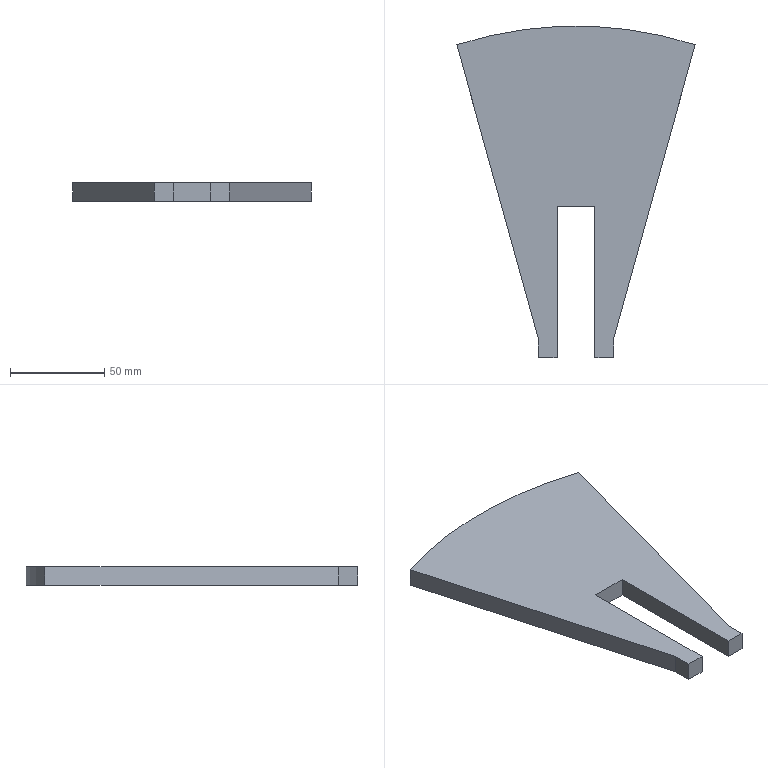Part | SolidWorks | features Extrusion 1, ICE 1 | 1 solid | 12 faces | box 126.548 x 176 x 10 mm | volume 126385 mm3 | plane 11 | cylinder 1 | commonest cylinder face diameters 412 x1
STEP:
#1=CARTESIAN_POINT('',(-20.,30.,-5.));
#2=VERTEX_POINT('',#1);
#3=CARTESIAN_POINT('',(-10.,30.,-5.));
#4=VERTEX_POINT('',#3);
#5=CARTESIAN_POINT('',(-20.,30.,-5.));
#6=DIRECTION('',(1.,0.,0.));
#7=VECTOR('',#6,1000.);
#8=LINE('',#5,#7);
#9=EDGE_CURVE('',#2,#4,#8,.T.);
#10=ORIENTED_EDGE('',*,*,#9,.T.);
#11=CARTESIAN_POINT('',(-10.,30.,5.));
#12=VERTEX_POINT('',#11);
#13=CARTESIAN_POINT('',(-10.,30.,5.));
#14=DIRECTION('',(0.,0.,1.));
#15=VECTOR('',#14,1000.);
#16=LINE('',#13,#15);
#17=EDGE_CURVE('',#4,#12,#16,.T.);
#18=ORIENTED_EDGE('',*,*,#17,.T.);
#19=CARTESIAN_POINT('',(-20.,30.,5.));
#20=VERTEX_POINT('',#19);
#21=CARTESIAN_POINT('',(-20.,30.,5.));
#22=DIRECTION('',(1.,0.,0.));
#23=VECTOR('',#22,1000.);
#24=LINE('',#21,#23);
#25=EDGE_CURVE('',#20,#12,#24,.T.);
#26=ORIENTED_EDGE('',*,*,#25,.F.);
#27=CARTESIAN_POINT('',(-20.,30.,5.));
#28=DIRECTION('',(0.,0.,-1.));
#29=VECTOR('',#28,1000.);
#30=LINE('',#27,#29);
#31=EDGE_CURVE('',#20,#2,#30,.T.);
#32=ORIENTED_EDGE('',*,*,#31,.T.);
#33=EDGE_LOOP('',(#10,#18,#26,#32));
#34=FACE_OUTER_BOUND('',#33,.T.);
#35=CARTESIAN_POINT('',(-20.,30.,5.));
#36=DIRECTION('',(0.,1.,0.));
#37=DIRECTION('',(-1.,0.,0.));
#38=AXIS2_PLACEMENT_3D('',#35,#36,#37);
#39=PLANE('',#38);
#40=ADVANCED_FACE('',(#34),#39,.F.);
#41=CARTESIAN_POINT('',(63.274,196.042,-5.));
#42=VERTEX_POINT('',#41);
#43=CARTESIAN_POINT('',(-63.274,196.042,-5.));
#44=VERTEX_POINT('',#43);
#45=CARTESIAN_POINT('',(0.,0.,-5.));
#46=DIRECTION('',(0.,0.,1.));
#47=DIRECTION('',(1.,0.,0.));
#48=AXIS2_PLACEMENT_3D('',#45,#46,#47);
#49=CIRCLE('',#48,206.);
#50=EDGE_CURVE('',#42,#44,#49,.T.);
#51=ORIENTED_EDGE('',*,*,#50,.T.);
#52=CARTESIAN_POINT('',(-63.274,196.042,5.));
#53=VERTEX_POINT('',#52);
#54=CARTESIAN_POINT('',(-63.274,196.042,5.));
#55=DIRECTION('',(0.,0.,-1.));
#56=VECTOR('',#55,1000.);
#57=LINE('',#54,#56);
#58=EDGE_CURVE('',#53,#44,#57,.T.);
#59=ORIENTED_EDGE('',*,*,#58,.F.);
#60=CARTESIAN_POINT('',(63.274,196.042,5.));
#61=VERTEX_POINT('',#60);
#62=CARTESIAN_POINT('',(0.,0.,5.));
#63=DIRECTION('',(0.,0.,1.));
#64=DIRECTION('',(1.,0.,0.));
#65=AXIS2_PLACEMENT_3D('',#62,#63,#64);
#66=CIRCLE('',#65,206.);
#67=EDGE_CURVE('',#61,#53,#66,.T.);
#68=ORIENTED_EDGE('',*,*,#67,.F.);
#69=CARTESIAN_POINT('',(63.274,196.042,5.));
#70=DIRECTION('',(0.,0.,-1.));
#71=VECTOR('',#70,1000.);
#72=LINE('',#69,#71);
#73=EDGE_CURVE('',#61,#42,#72,.T.);
#74=ORIENTED_EDGE('',*,*,#73,.T.);
#75=EDGE_LOOP('',(#51,#59,#68,#74));
#76=FACE_OUTER_BOUND('',#75,.T.);
#77=CARTESIAN_POINT('',(0.,0.,5.));
#78=DIRECTION('',(0.,0.,-1.));
#79=DIRECTION('',(-1.,0.,0.));
#80=AXIS2_PLACEMENT_3D('',#77,#78,#79);
#81=CYLINDRICAL_SURFACE('',#80,206.);
#82=ADVANCED_FACE('',(#76),#81,.T.);
#83=CARTESIAN_POINT('',(-20.,40.,-5.));
#84=VERTEX_POINT('',#83);
#85=CARTESIAN_POINT('',(-63.274,196.042,-5.));
#86=DIRECTION('',(0.2672,-0.9636,0.));
#87=VECTOR('',#86,1000.);
#88=LINE('',#85,#87);
#89=EDGE_CURVE('',#44,#84,#88,.T.);
#90=ORIENTED_EDGE('',*,*,#89,.T.);
#91=CARTESIAN_POINT('',(-20.,40.,5.));
#92=VERTEX_POINT('',#91);
#93=CARTESIAN_POINT('',(-20.,40.,5.));
#94=DIRECTION('',(0.,0.,-1.));
#95=VECTOR('',#94,1000.);
#96=LINE('',#93,#95);
#97=EDGE_CURVE('',#92,#84,#96,.T.);
#98=ORIENTED_EDGE('',*,*,#97,.F.);
#99=CARTESIAN_POINT('',(-63.274,196.042,5.));
#100=DIRECTION('',(0.2672,-0.9636,0.));
#101=VECTOR('',#100,1000.);
#102=LINE('',#99,#101);
#103=EDGE_CURVE('',#53,#92,#102,.T.);
#104=ORIENTED_EDGE('',*,*,#103,.F.);
#105=ORIENTED_EDGE('',*,*,#58,.T.);
#106=EDGE_LOOP('',(#90,#98,#104,#105));
#107=FACE_OUTER_BOUND('',#106,.T.);
#108=CARTESIAN_POINT('',(-63.274,196.042,5.));
#109=DIRECTION('',(0.9636,0.2672,0.));
#110=DIRECTION('',(-0.2672,0.9636,0.));
#111=AXIS2_PLACEMENT_3D('',#108,#109,#110);
#112=PLANE('',#111);
#113=ADVANCED_FACE('',(#107),#112,.F.);
#114=CARTESIAN_POINT('',(-20.,40.,-5.));
#115=DIRECTION('',(0.,-1.,0.));
#116=VECTOR('',#115,1000.);
#117=LINE('',#114,#116);
#118=EDGE_CURVE('',#84,#2,#117,.T.);
#119=ORIENTED_EDGE('',*,*,#118,.T.);
#120=ORIENTED_EDGE('',*,*,#31,.F.);
#121=CARTESIAN_POINT('',(-20.,40.,5.));
#122=DIRECTION('',(0.,-1.,0.));
#123=VECTOR('',#122,1000.);
#124=LINE('',#121,#123);
#125=EDGE_CURVE('',#92,#20,#124,.T.);
#126=ORIENTED_EDGE('',*,*,#125,.F.);
#127=ORIENTED_EDGE('',*,*,#97,.T.);
#128=EDGE_LOOP('',(#119,#120,#126,#127));
#129=FACE_OUTER_BOUND('',#128,.T.);
#130=CARTESIAN_POINT('',(-20.,40.,5.));
#131=DIRECTION('',(1.,0.,0.));
#132=DIRECTION('',(0.,0.,-1.));
#133=AXIS2_PLACEMENT_3D('',#130,#131,#132);
#134=PLANE('',#133);
#135=ADVANCED_FACE('',(#129),#134,.F.);
#136=CARTESIAN_POINT('',(10.,30.,5.));
#137=VERTEX_POINT('',#136);
#138=CARTESIAN_POINT('',(20.,30.,5.));
#139=VERTEX_POINT('',#138);
#140=CARTESIAN_POINT('',(-20.,30.,5.));
#141=DIRECTION('',(1.,0.,0.));
#142=VECTOR('',#141,1000.);
#143=LINE('',#140,#142);
#144=EDGE_CURVE('',#137,#139,#143,.T.);
#145=ORIENTED_EDGE('',*,*,#144,.F.);
#146=CARTESIAN_POINT('',(10.,30.,-5.));
#147=VERTEX_POINT('',#146);
#148=CARTESIAN_POINT('',(10.,30.,5.));
#149=DIRECTION('',(0.,0.,-1.));
#150=VECTOR('',#149,1000.);
#151=LINE('',#148,#150);
#152=EDGE_CURVE('',#137,#147,#151,.T.);
#153=ORIENTED_EDGE('',*,*,#152,.T.);
#154=CARTESIAN_POINT('',(20.,30.,-5.));
#155=VERTEX_POINT('',#154);
#156=CARTESIAN_POINT('',(-20.,30.,-5.));
#157=DIRECTION('',(1.,0.,0.));
#158=VECTOR('',#157,1000.);
#159=LINE('',#156,#158);
#160=EDGE_CURVE('',#147,#155,#159,.T.);
#161=ORIENTED_EDGE('',*,*,#160,.T.);
#162=CARTESIAN_POINT('',(20.,30.,5.));
#163=DIRECTION('',(0.,0.,-1.));
#164=VECTOR('',#163,1000.);
#165=LINE('',#162,#164);
#166=EDGE_CURVE('',#139,#155,#165,.T.);
#167=ORIENTED_EDGE('',*,*,#166,.F.);
#168=EDGE_LOOP('',(#145,#153,#161,#167));
#169=FACE_OUTER_BOUND('',#168,.T.);
#170=CARTESIAN_POINT('',(-20.,30.,5.));
#171=DIRECTION('',(0.,1.,0.));
#172=DIRECTION('',(-1.,0.,0.));
#173=AXIS2_PLACEMENT_3D('',#170,#171,#172);
#174=PLANE('',#173);
#175=ADVANCED_FACE('',(#169),#174,.F.);
#176=CARTESIAN_POINT('',(20.,40.,-5.));
#177=VERTEX_POINT('',#176);
#178=CARTESIAN_POINT('',(20.,30.,-5.));
#179=DIRECTION('',(0.,1.,0.));
#180=VECTOR('',#179,1000.);
#181=LINE('',#178,#180);
#182=EDGE_CURVE('',#155,#177,#181,.T.);
#183=ORIENTED_EDGE('',*,*,#182,.T.);
#184=CARTESIAN_POINT('',(20.,40.,5.));
#185=VERTEX_POINT('',#184);
#186=CARTESIAN_POINT('',(20.,40.,5.));
#187=DIRECTION('',(0.,0.,-1.));
#188=VECTOR('',#187,1000.);
#189=LINE('',#186,#188);
#190=EDGE_CURVE('',#185,#177,#189,.T.);
#191=ORIENTED_EDGE('',*,*,#190,.F.);
#192=CARTESIAN_POINT('',(20.,30.,5.));
#193=DIRECTION('',(0.,1.,0.));
#194=VECTOR('',#193,1000.);
#195=LINE('',#192,#194);
#196=EDGE_CURVE('',#139,#185,#195,.T.);
#197=ORIENTED_EDGE('',*,*,#196,.F.);
#198=ORIENTED_EDGE('',*,*,#166,.T.);
#199=EDGE_LOOP('',(#183,#191,#197,#198));
#200=FACE_OUTER_BOUND('',#199,.T.);
#201=CARTESIAN_POINT('',(20.,30.,5.));
#202=DIRECTION('',(-1.,0.,0.));
#203=DIRECTION('',(0.,-1.,0.));
#204=AXIS2_PLACEMENT_3D('',#201,#202,#203);
#205=PLANE('',#204);
#206=ADVANCED_FACE('',(#200),#205,.F.);
#207=CARTESIAN_POINT('',(20.,40.,-5.));
#208=DIRECTION('',(0.2672,0.9636,0.));
#209=VECTOR('',#208,1000.);
#210=LINE('',#207,#209);
#211=EDGE_CURVE('',#177,#42,#210,.T.);
#212=ORIENTED_EDGE('',*,*,#211,.T.);
#213=ORIENTED_EDGE('',*,*,#73,.F.);
#214=CARTESIAN_POINT('',(20.,40.,5.));
#215=DIRECTION('',(0.2672,0.9636,0.));
#216=VECTOR('',#215,1000.);
#217=LINE('',#214,#216);
#218=EDGE_CURVE('',#185,#61,#217,.T.);
#219=ORIENTED_EDGE('',*,*,#218,.F.);
#220=ORIENTED_EDGE('',*,*,#190,.T.);
#221=EDGE_LOOP('',(#212,#213,#219,#220));
#222=FACE_OUTER_BOUND('',#221,.T.);
#223=CARTESIAN_POINT('',(20.,40.,5.));
#224=DIRECTION('',(-0.9636,0.2672,0.));
#225=DIRECTION('',(-0.2672,-0.9636,0.));
#226=AXIS2_PLACEMENT_3D('',#223,#224,#225);
#227=PLANE('',#226);
#228=ADVANCED_FACE('',(#222),#227,.F.);
#229=CARTESIAN_POINT('',(-10.,110.,5.));
#230=VERTEX_POINT('',#229);
#231=CARTESIAN_POINT('',(-10.,-50.,5.));
#232=DIRECTION('',(0.,-1.,0.));
#233=VECTOR('',#232,1000.);
#234=LINE('',#231,#233);
#235=EDGE_CURVE('',#230,#12,#234,.T.);
#236=ORIENTED_EDGE('',*,*,#235,.F.);
#237=CARTESIAN_POINT('',(10.,110.,5.));
#238=VERTEX_POINT('',#237);
#239=CARTESIAN_POINT('',(10.,110.,5.));
#240=DIRECTION('',(-1.,0.,0.));
#241=VECTOR('',#240,1000.);
#242=LINE('',#239,#241);
#243=EDGE_CURVE('',#238,#230,#242,.T.);
#244=ORIENTED_EDGE('',*,*,#243,.F.);
#245=CARTESIAN_POINT('',(10.,-50.,5.));
#246=DIRECTION('',(0.,1.,0.));
#247=VECTOR('',#246,1000.);
#248=LINE('',#245,#247);
#249=EDGE_CURVE('',#137,#238,#248,.T.);
#250=ORIENTED_EDGE('',*,*,#249,.F.);
#251=ORIENTED_EDGE('',*,*,#144,.T.);
#252=ORIENTED_EDGE('',*,*,#196,.T.);
#253=ORIENTED_EDGE('',*,*,#218,.T.);
#254=ORIENTED_EDGE('',*,*,#67,.T.);
#255=ORIENTED_EDGE('',*,*,#103,.T.);
#256=ORIENTED_EDGE('',*,*,#125,.T.);
#257=ORIENTED_EDGE('',*,*,#25,.T.);
#258=EDGE_LOOP('',(#236,#244,#250,#251,#252,#253,#254,#255,#256,#257));
#259=FACE_OUTER_BOUND('',#258,.T.);
#260=CARTESIAN_POINT('',(0.,0.,5.));
#261=DIRECTION('',(0.,0.,1.));
#262=DIRECTION('',(1.,0.,0.));
#263=AXIS2_PLACEMENT_3D('',#260,#261,#262);
#264=PLANE('',#263);
#265=ADVANCED_FACE('',(#259),#264,.T.);
#266=CARTESIAN_POINT('',(10.,110.,-5.));
#267=VERTEX_POINT('',#266);
#268=CARTESIAN_POINT('',(-10.,110.,-5.));
#269=VERTEX_POINT('',#268);
#270=CARTESIAN_POINT('',(10.,110.,-5.));
#271=DIRECTION('',(-1.,0.,0.));
#272=VECTOR('',#271,1000.);
#273=LINE('',#270,#272);
#274=EDGE_CURVE('',#267,#269,#273,.T.);
#275=ORIENTED_EDGE('',*,*,#274,.T.);
#276=CARTESIAN_POINT('',(-10.,-50.,-5.));
#277=DIRECTION('',(0.,-1.,0.));
#278=VECTOR('',#277,1000.);
#279=LINE('',#276,#278);
#280=EDGE_CURVE('',#269,#4,#279,.T.);
#281=ORIENTED_EDGE('',*,*,#280,.T.);
#282=ORIENTED_EDGE('',*,*,#9,.F.);
#283=ORIENTED_EDGE('',*,*,#118,.F.);
#284=ORIENTED_EDGE('',*,*,#89,.F.);
#285=ORIENTED_EDGE('',*,*,#50,.F.);
#286=ORIENTED_EDGE('',*,*,#211,.F.);
#287=ORIENTED_EDGE('',*,*,#182,.F.);
#288=ORIENTED_EDGE('',*,*,#160,.F.);
#289=CARTESIAN_POINT('',(10.,0.,-5.));
#290=DIRECTION('',(0.,1.,0.));
#291=VECTOR('',#290,1000.);
#292=LINE('',#289,#291);
#293=EDGE_CURVE('',#147,#267,#292,.T.);
#294=ORIENTED_EDGE('',*,*,#293,.T.);
#295=EDGE_LOOP('',(#275,#281,#282,#283,#284,#285,#286,#287,#288,#294));
#296=FACE_OUTER_BOUND('',#295,.T.);
#297=CARTESIAN_POINT('',(0.,0.,-5.));
#298=DIRECTION('',(0.,0.,1.));
#299=DIRECTION('',(1.,0.,0.));
#300=AXIS2_PLACEMENT_3D('',#297,#298,#299);
#301=PLANE('',#300);
#302=ADVANCED_FACE('',(#296),#301,.F.);
#303=ORIENTED_EDGE('',*,*,#280,.F.);
#304=CARTESIAN_POINT('',(-10.,110.,-5.));
#305=DIRECTION('',(0.,0.,1.));
#306=VECTOR('',#305,1000.);
#307=LINE('',#304,#306);
#308=EDGE_CURVE('',#269,#230,#307,.T.);
#309=ORIENTED_EDGE('',*,*,#308,.T.);
#310=ORIENTED_EDGE('',*,*,#235,.T.);
#311=ORIENTED_EDGE('',*,*,#17,.F.);
#312=EDGE_LOOP('',(#303,#309,#310,#311));
#313=FACE_OUTER_BOUND('',#312,.T.);
#314=CARTESIAN_POINT('',(-10.,-50.,-5.));
#315=DIRECTION('',(-1.,0.,0.));
#316=DIRECTION('',(0.,0.,1.));
#317=AXIS2_PLACEMENT_3D('',#314,#315,#316);
#318=PLANE('',#317);
#319=ADVANCED_FACE('',(#313),#318,.F.);
#320=ORIENTED_EDGE('',*,*,#249,.T.);
#321=CARTESIAN_POINT('',(10.,110.,-5.));
#322=DIRECTION('',(0.,0.,1.));
#323=VECTOR('',#322,1000.);
#324=LINE('',#321,#323);
#325=EDGE_CURVE('',#267,#238,#324,.T.);
#326=ORIENTED_EDGE('',*,*,#325,.F.);
#327=ORIENTED_EDGE('',*,*,#293,.F.);
#328=ORIENTED_EDGE('',*,*,#152,.F.);
#329=EDGE_LOOP('',(#320,#326,#327,#328));
#330=FACE_OUTER_BOUND('',#329,.T.);
#331=CARTESIAN_POINT('',(10.,-50.,-5.));
#332=DIRECTION('',(1.,0.,0.));
#333=DIRECTION('',(0.,0.,-1.));
#334=AXIS2_PLACEMENT_3D('',#331,#332,#333);
#335=PLANE('',#334);
#336=ADVANCED_FACE('',(#330),#335,.F.);
#337=ORIENTED_EDGE('',*,*,#243,.T.);
#338=ORIENTED_EDGE('',*,*,#308,.F.);
#339=ORIENTED_EDGE('',*,*,#274,.F.);
#340=ORIENTED_EDGE('',*,*,#325,.T.);
#341=EDGE_LOOP('',(#337,#338,#339,#340));
#342=FACE_OUTER_BOUND('',#341,.T.);
#343=CARTESIAN_POINT('',(10.,110.,-5.));
#344=DIRECTION('',(0.,1.,0.));
#345=DIRECTION('',(-1.,0.,0.));
#346=AXIS2_PLACEMENT_3D('',#343,#344,#345);
#347=PLANE('',#346);
#348=ADVANCED_FACE('',(#342),#347,.F.);
#349=CLOSED_SHELL('',(#40,#82,#113,#135,#175,#206,#228,#265,#302,#319,#336,#348));
#350=MANIFOLD_SOLID_BREP('',#349);
#351=CARTESIAN_POINT('',(0.,0.,0.));
#352=DIRECTION('',(0.,0.,1.));
#353=DIRECTION('',(1.,0.,0.));
#354=AXIS2_PLACEMENT_3D('',#351,#352,#353);
#355=(LENGTH_UNIT()NAMED_UNIT(*)SI_UNIT(.MILLI.,.METRE.));
#356=UNCERTAINTY_MEASURE_WITH_UNIT(LENGTH_MEASURE(0.00001),#355,'','');
#357=(NAMED_UNIT(*)PLANE_ANGLE_UNIT()SI_UNIT($,.RADIAN.));
#358=(NAMED_UNIT(*)SI_UNIT($,.STERADIAN.)SOLID_ANGLE_UNIT());
#359=(GEOMETRIC_REPRESENTATION_CONTEXT(3)GLOBAL_UNCERTAINTY_ASSIGNED_CONTEXT((#356))GLOBAL_UNIT_ASSIGNED_CONTEXT((#355,#357,#358))REPRESENTATION_CONTEXT('',''));
#360=ADVANCED_BREP_SHAPE_REPRESENTATION('',(#350,#354),#359);